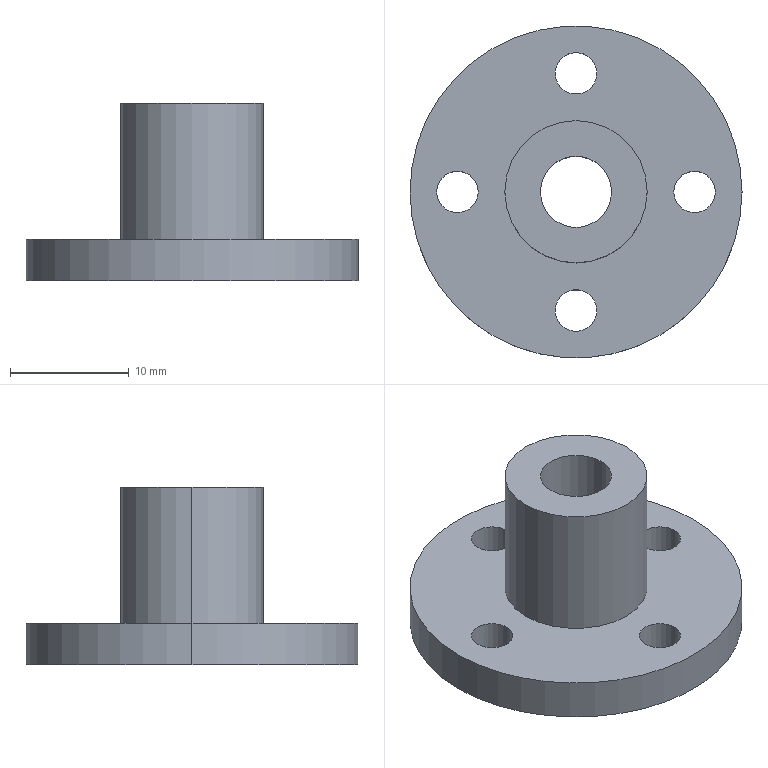Part | SolidWorks | features ICE 3, CirPattern 1, Extrusion 1 | 1 solid | 17 faces | box 28 x 28 x 15 mm | volume 2897 mm3 | cylinder 14 | plane 3 | commonest cylinder face diameters 3.5 x8 6 x2 12 x2 28 x2
STEP:
#1=CARTESIAN_POINT('',(-3.,0.,0.));
#2=VERTEX_POINT('',#1);
#3=CARTESIAN_POINT('',(3.,0.,0.));
#4=VERTEX_POINT('',#3);
#5=CARTESIAN_POINT('',(0.,0.,0.));
#6=DIRECTION('',(0.,0.,1.));
#7=DIRECTION('',(1.,0.,0.));
#8=AXIS2_PLACEMENT_3D('',#5,#6,#7);
#9=CIRCLE('',#8,3.);
#10=EDGE_CURVE('',#2,#4,#9,.T.);
#11=ORIENTED_EDGE('',*,*,#10,.F.);
#12=CARTESIAN_POINT('',(-3.,0.,15.));
#13=VERTEX_POINT('',#12);
#14=CARTESIAN_POINT('',(-3.,0.,-35.));
#15=DIRECTION('',(0.,0.,1.));
#16=VECTOR('',#15,1000.);
#17=LINE('',#14,#16);
#18=EDGE_CURVE('',#2,#13,#17,.T.);
#19=ORIENTED_EDGE('',*,*,#18,.T.);
#20=CARTESIAN_POINT('',(3.,0.,15.));
#21=VERTEX_POINT('',#20);
#22=CARTESIAN_POINT('',(0.,0.,15.));
#23=DIRECTION('',(0.,0.,1.));
#24=DIRECTION('',(1.,0.,0.));
#25=AXIS2_PLACEMENT_3D('',#22,#23,#24);
#26=CIRCLE('',#25,3.);
#27=EDGE_CURVE('',#13,#21,#26,.T.);
#28=ORIENTED_EDGE('',*,*,#27,.T.);
#29=CARTESIAN_POINT('',(3.,0.,-35.));
#30=DIRECTION('',(0.,0.,1.));
#31=VECTOR('',#30,1000.);
#32=LINE('',#29,#31);
#33=EDGE_CURVE('',#4,#21,#32,.T.);
#34=ORIENTED_EDGE('',*,*,#33,.F.);
#35=EDGE_LOOP('',(#11,#19,#28,#34));
#36=FACE_OUTER_BOUND('',#35,.T.);
#37=CARTESIAN_POINT('',(0.,0.,-35.));
#38=DIRECTION('',(0.,0.,1.));
#39=DIRECTION('',(1.,0.,0.));
#40=AXIS2_PLACEMENT_3D('',#37,#38,#39);
#41=CYLINDRICAL_SURFACE('',#40,3.);
#42=ADVANCED_FACE('',(#36),#41,.F.);
#43=CARTESIAN_POINT('',(-11.75,0.,0.));
#44=VERTEX_POINT('',#43);
#45=CARTESIAN_POINT('',(-8.25,0.,0.));
#46=VERTEX_POINT('',#45);
#47=CARTESIAN_POINT('',(-10.,0.,0.));
#48=DIRECTION('',(0.,0.,1.));
#49=DIRECTION('',(1.,0.,0.));
#50=AXIS2_PLACEMENT_3D('',#47,#48,#49);
#51=CIRCLE('',#50,1.75);
#52=EDGE_CURVE('',#44,#46,#51,.T.);
#53=ORIENTED_EDGE('',*,*,#52,.F.);
#54=CARTESIAN_POINT('',(-11.75,0.,3.5));
#55=VERTEX_POINT('',#54);
#56=CARTESIAN_POINT('',(-11.75,0.,-8.));
#57=DIRECTION('',(0.,0.,1.));
#58=VECTOR('',#57,1000.);
#59=LINE('',#56,#58);
#60=EDGE_CURVE('',#44,#55,#59,.T.);
#61=ORIENTED_EDGE('',*,*,#60,.T.);
#62=CARTESIAN_POINT('',(-8.25,0.,3.5));
#63=VERTEX_POINT('',#62);
#64=CARTESIAN_POINT('',(-10.,0.,3.5));
#65=DIRECTION('',(0.,0.,1.));
#66=DIRECTION('',(0.,1.,0.));
#67=AXIS2_PLACEMENT_3D('',#64,#65,#66);
#68=CIRCLE('',#67,1.75);
#69=EDGE_CURVE('',#55,#63,#68,.T.);
#70=ORIENTED_EDGE('',*,*,#69,.T.);
#71=CARTESIAN_POINT('',(-8.25,0.,-8.));
#72=DIRECTION('',(0.,0.,1.));
#73=VECTOR('',#72,1000.);
#74=LINE('',#71,#73);
#75=EDGE_CURVE('',#46,#63,#74,.T.);
#76=ORIENTED_EDGE('',*,*,#75,.F.);
#77=EDGE_LOOP('',(#53,#61,#70,#76));
#78=FACE_OUTER_BOUND('',#77,.T.);
#79=CARTESIAN_POINT('',(-10.,0.,-8.));
#80=DIRECTION('',(0.,0.,1.));
#81=DIRECTION('',(1.,0.,0.));
#82=AXIS2_PLACEMENT_3D('',#79,#80,#81);
#83=CYLINDRICAL_SURFACE('',#82,1.75);
#84=ADVANCED_FACE('',(#78),#83,.F.);
#85=CARTESIAN_POINT('',(-1.75,-10.,0.));
#86=VERTEX_POINT('',#85);
#87=CARTESIAN_POINT('',(1.75,-10.,0.));
#88=VERTEX_POINT('',#87);
#89=CARTESIAN_POINT('',(0.,-10.,0.));
#90=DIRECTION('',(0.,0.,1.));
#91=DIRECTION('',(1.,0.,0.));
#92=AXIS2_PLACEMENT_3D('',#89,#90,#91);
#93=CIRCLE('',#92,1.75);
#94=EDGE_CURVE('',#86,#88,#93,.T.);
#95=ORIENTED_EDGE('',*,*,#94,.F.);
#96=CARTESIAN_POINT('',(-1.75,-10.,3.5));
#97=VERTEX_POINT('',#96);
#98=CARTESIAN_POINT('',(-1.75,-10.,-8.));
#99=DIRECTION('',(0.,0.,1.));
#100=VECTOR('',#99,1000.);
#101=LINE('',#98,#100);
#102=EDGE_CURVE('',#86,#97,#101,.T.);
#103=ORIENTED_EDGE('',*,*,#102,.T.);
#104=CARTESIAN_POINT('',(1.75,-10.,3.5));
#105=VERTEX_POINT('',#104);
#106=CARTESIAN_POINT('',(0.,-10.,3.5));
#107=DIRECTION('',(0.,0.,1.));
#108=DIRECTION('',(-1.,0.,0.));
#109=AXIS2_PLACEMENT_3D('',#106,#107,#108);
#110=CIRCLE('',#109,1.75);
#111=EDGE_CURVE('',#97,#105,#110,.T.);
#112=ORIENTED_EDGE('',*,*,#111,.T.);
#113=CARTESIAN_POINT('',(1.75,-10.,-8.));
#114=DIRECTION('',(0.,0.,1.));
#115=VECTOR('',#114,1000.);
#116=LINE('',#113,#115);
#117=EDGE_CURVE('',#88,#105,#116,.T.);
#118=ORIENTED_EDGE('',*,*,#117,.F.);
#119=EDGE_LOOP('',(#95,#103,#112,#118));
#120=FACE_OUTER_BOUND('',#119,.T.);
#121=CARTESIAN_POINT('',(0.,-10.,-8.));
#122=DIRECTION('',(0.,0.,1.));
#123=DIRECTION('',(1.,0.,0.));
#124=AXIS2_PLACEMENT_3D('',#121,#122,#123);
#125=CYLINDRICAL_SURFACE('',#124,1.75);
#126=ADVANCED_FACE('',(#120),#125,.F.);
#127=CARTESIAN_POINT('',(8.25,0.,0.));
#128=VERTEX_POINT('',#127);
#129=CARTESIAN_POINT('',(11.75,0.,0.));
#130=VERTEX_POINT('',#129);
#131=CARTESIAN_POINT('',(10.,0.,0.));
#132=DIRECTION('',(0.,0.,1.));
#133=DIRECTION('',(1.,0.,0.));
#134=AXIS2_PLACEMENT_3D('',#131,#132,#133);
#135=CIRCLE('',#134,1.75);
#136=EDGE_CURVE('',#128,#130,#135,.T.);
#137=ORIENTED_EDGE('',*,*,#136,.F.);
#138=CARTESIAN_POINT('',(8.25,0.,3.5));
#139=VERTEX_POINT('',#138);
#140=CARTESIAN_POINT('',(8.25,0.,-8.));
#141=DIRECTION('',(0.,0.,1.));
#142=VECTOR('',#141,1000.);
#143=LINE('',#140,#142);
#144=EDGE_CURVE('',#128,#139,#143,.T.);
#145=ORIENTED_EDGE('',*,*,#144,.T.);
#146=CARTESIAN_POINT('',(11.75,0.,3.5));
#147=VERTEX_POINT('',#146);
#148=CARTESIAN_POINT('',(10.,0.,3.5));
#149=DIRECTION('',(0.,0.,1.));
#150=DIRECTION('',(0.,-1.,0.));
#151=AXIS2_PLACEMENT_3D('',#148,#149,#150);
#152=CIRCLE('',#151,1.75);
#153=EDGE_CURVE('',#139,#147,#152,.T.);
#154=ORIENTED_EDGE('',*,*,#153,.T.);
#155=CARTESIAN_POINT('',(11.75,0.,-8.));
#156=DIRECTION('',(0.,0.,1.));
#157=VECTOR('',#156,1000.);
#158=LINE('',#155,#157);
#159=EDGE_CURVE('',#130,#147,#158,.T.);
#160=ORIENTED_EDGE('',*,*,#159,.F.);
#161=EDGE_LOOP('',(#137,#145,#154,#160));
#162=FACE_OUTER_BOUND('',#161,.T.);
#163=CARTESIAN_POINT('',(10.,0.,-8.));
#164=DIRECTION('',(0.,0.,1.));
#165=DIRECTION('',(1.,0.,0.));
#166=AXIS2_PLACEMENT_3D('',#163,#164,#165);
#167=CYLINDRICAL_SURFACE('',#166,1.75);
#168=ADVANCED_FACE('',(#162),#167,.F.);
#169=CARTESIAN_POINT('',(-1.75,10.,0.));
#170=VERTEX_POINT('',#169);
#171=CARTESIAN_POINT('',(1.75,10.,0.));
#172=VERTEX_POINT('',#171);
#173=CARTESIAN_POINT('',(0.,10.,0.));
#174=DIRECTION('',(0.,0.,1.));
#175=DIRECTION('',(1.,0.,0.));
#176=AXIS2_PLACEMENT_3D('',#173,#174,#175);
#177=CIRCLE('',#176,1.75);
#178=EDGE_CURVE('',#170,#172,#177,.T.);
#179=ORIENTED_EDGE('',*,*,#178,.F.);
#180=CARTESIAN_POINT('',(-1.75,10.,3.5));
#181=VERTEX_POINT('',#180);
#182=CARTESIAN_POINT('',(-1.75,10.,-8.));
#183=DIRECTION('',(0.,0.,1.));
#184=VECTOR('',#183,1000.);
#185=LINE('',#182,#184);
#186=EDGE_CURVE('',#170,#181,#185,.T.);
#187=ORIENTED_EDGE('',*,*,#186,.T.);
#188=CARTESIAN_POINT('',(1.75,10.,3.5));
#189=VERTEX_POINT('',#188);
#190=CARTESIAN_POINT('',(0.,10.,3.5));
#191=DIRECTION('',(0.,0.,1.));
#192=DIRECTION('',(1.,0.,0.));
#193=AXIS2_PLACEMENT_3D('',#190,#191,#192);
#194=CIRCLE('',#193,1.75);
#195=EDGE_CURVE('',#181,#189,#194,.T.);
#196=ORIENTED_EDGE('',*,*,#195,.T.);
#197=CARTESIAN_POINT('',(1.75,10.,-8.));
#198=DIRECTION('',(0.,0.,1.));
#199=VECTOR('',#198,1000.);
#200=LINE('',#197,#199);
#201=EDGE_CURVE('',#172,#189,#200,.T.);
#202=ORIENTED_EDGE('',*,*,#201,.F.);
#203=EDGE_LOOP('',(#179,#187,#196,#202));
#204=FACE_OUTER_BOUND('',#203,.T.);
#205=CARTESIAN_POINT('',(0.,10.,-8.));
#206=DIRECTION('',(0.,0.,1.));
#207=DIRECTION('',(1.,0.,0.));
#208=AXIS2_PLACEMENT_3D('',#205,#206,#207);
#209=CYLINDRICAL_SURFACE('',#208,1.75);
#210=ADVANCED_FACE('',(#204),#209,.F.);
#211=CARTESIAN_POINT('',(6.,0.,15.));
#212=VERTEX_POINT('',#211);
#213=CARTESIAN_POINT('',(-6.,0.,15.));
#214=VERTEX_POINT('',#213);
#215=CARTESIAN_POINT('',(0.,0.,15.));
#216=DIRECTION('',(0.,0.,1.));
#217=DIRECTION('',(1.,0.,0.));
#218=AXIS2_PLACEMENT_3D('',#215,#216,#217);
#219=CIRCLE('',#218,6.);
#220=EDGE_CURVE('',#212,#214,#219,.T.);
#221=ORIENTED_EDGE('',*,*,#220,.F.);
#222=CARTESIAN_POINT('',(6.,0.,3.5));
#223=VERTEX_POINT('',#222);
#224=CARTESIAN_POINT('',(6.,0.,15.));
#225=DIRECTION('',(0.,0.,-1.));
#226=VECTOR('',#225,1000.);
#227=LINE('',#224,#226);
#228=EDGE_CURVE('',#212,#223,#227,.T.);
#229=ORIENTED_EDGE('',*,*,#228,.T.);
#230=CARTESIAN_POINT('',(-6.,0.,3.5));
#231=VERTEX_POINT('',#230);
#232=CARTESIAN_POINT('',(0.,0.,3.5));
#233=DIRECTION('',(0.,0.,1.));
#234=DIRECTION('',(1.,0.,0.));
#235=AXIS2_PLACEMENT_3D('',#232,#233,#234);
#236=CIRCLE('',#235,6.);
#237=EDGE_CURVE('',#223,#231,#236,.T.);
#238=ORIENTED_EDGE('',*,*,#237,.T.);
#239=CARTESIAN_POINT('',(-6.,0.,15.));
#240=DIRECTION('',(0.,0.,-1.));
#241=VECTOR('',#240,1000.);
#242=LINE('',#239,#241);
#243=EDGE_CURVE('',#214,#231,#242,.T.);
#244=ORIENTED_EDGE('',*,*,#243,.F.);
#245=EDGE_LOOP('',(#221,#229,#238,#244));
#246=FACE_OUTER_BOUND('',#245,.T.);
#247=CARTESIAN_POINT('',(0.,0.,15.));
#248=DIRECTION('',(0.,0.,-1.));
#249=DIRECTION('',(-1.,0.,0.));
#250=AXIS2_PLACEMENT_3D('',#247,#248,#249);
#251=CYLINDRICAL_SURFACE('',#250,6.);
#252=ADVANCED_FACE('',(#246),#251,.T.);
#253=CARTESIAN_POINT('',(14.,0.,3.5));
#254=VERTEX_POINT('',#253);
#255=CARTESIAN_POINT('',(-14.,0.,3.5));
#256=VERTEX_POINT('',#255);
#257=CARTESIAN_POINT('',(0.,0.,3.5));
#258=DIRECTION('',(0.,0.,1.));
#259=DIRECTION('',(1.,0.,0.));
#260=AXIS2_PLACEMENT_3D('',#257,#258,#259);
#261=CIRCLE('',#260,14.);
#262=EDGE_CURVE('',#254,#256,#261,.T.);
#263=ORIENTED_EDGE('',*,*,#262,.F.);
#264=CARTESIAN_POINT('',(14.,0.,0.));
#265=VERTEX_POINT('',#264);
#266=CARTESIAN_POINT('',(14.,0.,3.5));
#267=DIRECTION('',(0.,0.,-1.));
#268=VECTOR('',#267,1000.);
#269=LINE('',#266,#268);
#270=EDGE_CURVE('',#254,#265,#269,.T.);
#271=ORIENTED_EDGE('',*,*,#270,.T.);
#272=CARTESIAN_POINT('',(-14.,0.,0.));
#273=VERTEX_POINT('',#272);
#274=CARTESIAN_POINT('',(0.,0.,0.));
#275=DIRECTION('',(0.,0.,1.));
#276=DIRECTION('',(1.,0.,0.));
#277=AXIS2_PLACEMENT_3D('',#274,#275,#276);
#278=CIRCLE('',#277,14.);
#279=EDGE_CURVE('',#265,#273,#278,.T.);
#280=ORIENTED_EDGE('',*,*,#279,.T.);
#281=CARTESIAN_POINT('',(-14.,0.,3.5));
#282=DIRECTION('',(0.,0.,-1.));
#283=VECTOR('',#282,1000.);
#284=LINE('',#281,#283);
#285=EDGE_CURVE('',#256,#273,#284,.T.);
#286=ORIENTED_EDGE('',*,*,#285,.F.);
#287=EDGE_LOOP('',(#263,#271,#280,#286));
#288=FACE_OUTER_BOUND('',#287,.T.);
#289=CARTESIAN_POINT('',(0.,0.,3.5));
#290=DIRECTION('',(0.,0.,-1.));
#291=DIRECTION('',(-1.,0.,0.));
#292=AXIS2_PLACEMENT_3D('',#289,#290,#291);
#293=CYLINDRICAL_SURFACE('',#292,14.);
#294=ADVANCED_FACE('',(#288),#293,.T.);
#295=ORIENTED_EDGE('',*,*,#270,.F.);
#296=CARTESIAN_POINT('',(0.,0.,3.5));
#297=DIRECTION('',(0.,0.,1.));
#298=DIRECTION('',(1.,0.,0.));
#299=AXIS2_PLACEMENT_3D('',#296,#297,#298);
#300=CIRCLE('',#299,14.);
#301=EDGE_CURVE('',#256,#254,#300,.T.);
#302=ORIENTED_EDGE('',*,*,#301,.F.);
#303=ORIENTED_EDGE('',*,*,#285,.T.);
#304=CARTESIAN_POINT('',(0.,0.,0.));
#305=DIRECTION('',(0.,0.,1.));
#306=DIRECTION('',(1.,0.,0.));
#307=AXIS2_PLACEMENT_3D('',#304,#305,#306);
#308=CIRCLE('',#307,14.);
#309=EDGE_CURVE('',#273,#265,#308,.T.);
#310=ORIENTED_EDGE('',*,*,#309,.T.);
#311=EDGE_LOOP('',(#295,#302,#303,#310));
#312=FACE_OUTER_BOUND('',#311,.T.);
#313=CARTESIAN_POINT('',(0.,0.,3.5));
#314=DIRECTION('',(0.,0.,-1.));
#315=DIRECTION('',(-1.,0.,0.));
#316=AXIS2_PLACEMENT_3D('',#313,#314,#315);
#317=CYLINDRICAL_SURFACE('',#316,14.);
#318=ADVANCED_FACE('',(#312),#317,.T.);
#319=CARTESIAN_POINT('',(-10.,0.,3.5));
#320=DIRECTION('',(0.,0.,1.));
#321=DIRECTION('',(0.,1.,0.));
#322=AXIS2_PLACEMENT_3D('',#319,#320,#321);
#323=CIRCLE('',#322,1.75);
#324=EDGE_CURVE('',#63,#55,#323,.T.);
#325=ORIENTED_EDGE('',*,*,#324,.F.);
#326=ORIENTED_EDGE('',*,*,#69,.F.);
#327=EDGE_LOOP('',(#325,#326));
#328=FACE_BOUND('',#327,.T.);
#329=CARTESIAN_POINT('',(0.,-10.,3.5));
#330=DIRECTION('',(0.,0.,1.));
#331=DIRECTION('',(-1.,0.,0.));
#332=AXIS2_PLACEMENT_3D('',#329,#330,#331);
#333=CIRCLE('',#332,1.75);
#334=EDGE_CURVE('',#105,#97,#333,.T.);
#335=ORIENTED_EDGE('',*,*,#334,.F.);
#336=ORIENTED_EDGE('',*,*,#111,.F.);
#337=EDGE_LOOP('',(#335,#336));
#338=FACE_BOUND('',#337,.T.);
#339=CARTESIAN_POINT('',(10.,0.,3.5));
#340=DIRECTION('',(0.,0.,1.));
#341=DIRECTION('',(0.,-1.,0.));
#342=AXIS2_PLACEMENT_3D('',#339,#340,#341);
#343=CIRCLE('',#342,1.75);
#344=EDGE_CURVE('',#147,#139,#343,.T.);
#345=ORIENTED_EDGE('',*,*,#344,.F.);
#346=ORIENTED_EDGE('',*,*,#153,.F.);
#347=EDGE_LOOP('',(#345,#346));
#348=FACE_BOUND('',#347,.T.);
#349=CARTESIAN_POINT('',(0.,10.,3.5));
#350=DIRECTION('',(0.,0.,1.));
#351=DIRECTION('',(1.,0.,0.));
#352=AXIS2_PLACEMENT_3D('',#349,#350,#351);
#353=CIRCLE('',#352,1.75);
#354=EDGE_CURVE('',#189,#181,#353,.T.);
#355=ORIENTED_EDGE('',*,*,#354,.F.);
#356=ORIENTED_EDGE('',*,*,#195,.F.);
#357=EDGE_LOOP('',(#355,#356));
#358=FACE_BOUND('',#357,.T.);
#359=CARTESIAN_POINT('',(0.,0.,3.5));
#360=DIRECTION('',(0.,0.,1.));
#361=DIRECTION('',(1.,0.,0.));
#362=AXIS2_PLACEMENT_3D('',#359,#360,#361);
#363=CIRCLE('',#362,6.);
#364=EDGE_CURVE('',#231,#223,#363,.T.);
#365=ORIENTED_EDGE('',*,*,#364,.F.);
#366=ORIENTED_EDGE('',*,*,#237,.F.);
#367=EDGE_LOOP('',(#365,#366));
#368=FACE_BOUND('',#367,.T.);
#369=ORIENTED_EDGE('',*,*,#301,.T.);
#370=ORIENTED_EDGE('',*,*,#262,.T.);
#371=EDGE_LOOP('',(#369,#370));
#372=FACE_OUTER_BOUND('',#371,.T.);
#373=CARTESIAN_POINT('',(0.,0.,3.5));
#374=DIRECTION('',(0.,0.,1.));
#375=DIRECTION('',(1.,0.,0.));
#376=AXIS2_PLACEMENT_3D('',#373,#374,#375);
#377=PLANE('',#376);
#378=ADVANCED_FACE('',(#328,#338,#348,#358,#368,#372),#377,.T.);
#379=CARTESIAN_POINT('',(0.,0.,0.));
#380=DIRECTION('',(0.,0.,1.));
#381=DIRECTION('',(1.,0.,0.));
#382=AXIS2_PLACEMENT_3D('',#379,#380,#381);
#383=CIRCLE('',#382,3.);
#384=EDGE_CURVE('',#4,#2,#383,.T.);
#385=ORIENTED_EDGE('',*,*,#384,.T.);
#386=ORIENTED_EDGE('',*,*,#10,.T.);
#387=EDGE_LOOP('',(#385,#386));
#388=FACE_BOUND('',#387,.T.);
#389=CARTESIAN_POINT('',(-10.,0.,0.));
#390=DIRECTION('',(0.,0.,1.));
#391=DIRECTION('',(1.,0.,0.));
#392=AXIS2_PLACEMENT_3D('',#389,#390,#391);
#393=CIRCLE('',#392,1.75);
#394=EDGE_CURVE('',#46,#44,#393,.T.);
#395=ORIENTED_EDGE('',*,*,#394,.T.);
#396=ORIENTED_EDGE('',*,*,#52,.T.);
#397=EDGE_LOOP('',(#395,#396));
#398=FACE_BOUND('',#397,.T.);
#399=CARTESIAN_POINT('',(0.,-10.,0.));
#400=DIRECTION('',(0.,0.,1.));
#401=DIRECTION('',(1.,0.,0.));
#402=AXIS2_PLACEMENT_3D('',#399,#400,#401);
#403=CIRCLE('',#402,1.75);
#404=EDGE_CURVE('',#88,#86,#403,.T.);
#405=ORIENTED_EDGE('',*,*,#404,.T.);
#406=ORIENTED_EDGE('',*,*,#94,.T.);
#407=EDGE_LOOP('',(#405,#406));
#408=FACE_BOUND('',#407,.T.);
#409=CARTESIAN_POINT('',(10.,0.,0.));
#410=DIRECTION('',(0.,0.,1.));
#411=DIRECTION('',(1.,0.,0.));
#412=AXIS2_PLACEMENT_3D('',#409,#410,#411);
#413=CIRCLE('',#412,1.75);
#414=EDGE_CURVE('',#130,#128,#413,.T.);
#415=ORIENTED_EDGE('',*,*,#414,.T.);
#416=ORIENTED_EDGE('',*,*,#136,.T.);
#417=EDGE_LOOP('',(#415,#416));
#418=FACE_BOUND('',#417,.T.);
#419=CARTESIAN_POINT('',(0.,10.,0.));
#420=DIRECTION('',(0.,0.,1.));
#421=DIRECTION('',(1.,0.,0.));
#422=AXIS2_PLACEMENT_3D('',#419,#420,#421);
#423=CIRCLE('',#422,1.75);
#424=EDGE_CURVE('',#172,#170,#423,.T.);
#425=ORIENTED_EDGE('',*,*,#424,.T.);
#426=ORIENTED_EDGE('',*,*,#178,.T.);
#427=EDGE_LOOP('',(#425,#426));
#428=FACE_BOUND('',#427,.T.);
#429=ORIENTED_EDGE('',*,*,#309,.F.);
#430=ORIENTED_EDGE('',*,*,#279,.F.);
#431=EDGE_LOOP('',(#429,#430));
#432=FACE_OUTER_BOUND('',#431,.T.);
#433=CARTESIAN_POINT('',(0.,0.,0.));
#434=DIRECTION('',(0.,0.,1.));
#435=DIRECTION('',(1.,0.,0.));
#436=AXIS2_PLACEMENT_3D('',#433,#434,#435);
#437=PLANE('',#436);
#438=ADVANCED_FACE('',(#388,#398,#408,#418,#428,#432),#437,.F.);
#439=ORIENTED_EDGE('',*,*,#228,.F.);
#440=CARTESIAN_POINT('',(0.,0.,15.));
#441=DIRECTION('',(0.,0.,1.));
#442=DIRECTION('',(1.,0.,0.));
#443=AXIS2_PLACEMENT_3D('',#440,#441,#442);
#444=CIRCLE('',#443,6.);
#445=EDGE_CURVE('',#214,#212,#444,.T.);
#446=ORIENTED_EDGE('',*,*,#445,.F.);
#447=ORIENTED_EDGE('',*,*,#243,.T.);
#448=ORIENTED_EDGE('',*,*,#364,.T.);
#449=EDGE_LOOP('',(#439,#446,#447,#448));
#450=FACE_OUTER_BOUND('',#449,.T.);
#451=CARTESIAN_POINT('',(0.,0.,15.));
#452=DIRECTION('',(0.,0.,-1.));
#453=DIRECTION('',(-1.,0.,0.));
#454=AXIS2_PLACEMENT_3D('',#451,#452,#453);
#455=CYLINDRICAL_SURFACE('',#454,6.);
#456=ADVANCED_FACE('',(#450),#455,.T.);
#457=CARTESIAN_POINT('',(0.,0.,15.));
#458=DIRECTION('',(0.,0.,1.));
#459=DIRECTION('',(1.,0.,0.));
#460=AXIS2_PLACEMENT_3D('',#457,#458,#459);
#461=CIRCLE('',#460,3.);
#462=EDGE_CURVE('',#21,#13,#461,.T.);
#463=ORIENTED_EDGE('',*,*,#462,.F.);
#464=ORIENTED_EDGE('',*,*,#27,.F.);
#465=EDGE_LOOP('',(#463,#464));
#466=FACE_BOUND('',#465,.T.);
#467=ORIENTED_EDGE('',*,*,#445,.T.);
#468=ORIENTED_EDGE('',*,*,#220,.T.);
#469=EDGE_LOOP('',(#467,#468));
#470=FACE_OUTER_BOUND('',#469,.T.);
#471=CARTESIAN_POINT('',(0.,0.,15.));
#472=DIRECTION('',(0.,0.,1.));
#473=DIRECTION('',(1.,0.,0.));
#474=AXIS2_PLACEMENT_3D('',#471,#472,#473);
#475=PLANE('',#474);
#476=ADVANCED_FACE('',(#466,#470),#475,.T.);
#477=ORIENTED_EDGE('',*,*,#186,.F.);
#478=ORIENTED_EDGE('',*,*,#424,.F.);
#479=ORIENTED_EDGE('',*,*,#201,.T.);
#480=ORIENTED_EDGE('',*,*,#354,.T.);
#481=EDGE_LOOP('',(#477,#478,#479,#480));
#482=FACE_OUTER_BOUND('',#481,.T.);
#483=CARTESIAN_POINT('',(0.,10.,-8.));
#484=DIRECTION('',(0.,0.,1.));
#485=DIRECTION('',(1.,0.,0.));
#486=AXIS2_PLACEMENT_3D('',#483,#484,#485);
#487=CYLINDRICAL_SURFACE('',#486,1.75);
#488=ADVANCED_FACE('',(#482),#487,.F.);
#489=ORIENTED_EDGE('',*,*,#144,.F.);
#490=ORIENTED_EDGE('',*,*,#414,.F.);
#491=ORIENTED_EDGE('',*,*,#159,.T.);
#492=ORIENTED_EDGE('',*,*,#344,.T.);
#493=EDGE_LOOP('',(#489,#490,#491,#492));
#494=FACE_OUTER_BOUND('',#493,.T.);
#495=CARTESIAN_POINT('',(10.,0.,-8.));
#496=DIRECTION('',(0.,0.,1.));
#497=DIRECTION('',(1.,0.,0.));
#498=AXIS2_PLACEMENT_3D('',#495,#496,#497);
#499=CYLINDRICAL_SURFACE('',#498,1.75);
#500=ADVANCED_FACE('',(#494),#499,.F.);
#501=ORIENTED_EDGE('',*,*,#102,.F.);
#502=ORIENTED_EDGE('',*,*,#404,.F.);
#503=ORIENTED_EDGE('',*,*,#117,.T.);
#504=ORIENTED_EDGE('',*,*,#334,.T.);
#505=EDGE_LOOP('',(#501,#502,#503,#504));
#506=FACE_OUTER_BOUND('',#505,.T.);
#507=CARTESIAN_POINT('',(0.,-10.,-8.));
#508=DIRECTION('',(0.,0.,1.));
#509=DIRECTION('',(1.,0.,0.));
#510=AXIS2_PLACEMENT_3D('',#507,#508,#509);
#511=CYLINDRICAL_SURFACE('',#510,1.75);
#512=ADVANCED_FACE('',(#506),#511,.F.);
#513=ORIENTED_EDGE('',*,*,#60,.F.);
#514=ORIENTED_EDGE('',*,*,#394,.F.);
#515=ORIENTED_EDGE('',*,*,#75,.T.);
#516=ORIENTED_EDGE('',*,*,#324,.T.);
#517=EDGE_LOOP('',(#513,#514,#515,#516));
#518=FACE_OUTER_BOUND('',#517,.T.);
#519=CARTESIAN_POINT('',(-10.,0.,-8.));
#520=DIRECTION('',(0.,0.,1.));
#521=DIRECTION('',(1.,0.,0.));
#522=AXIS2_PLACEMENT_3D('',#519,#520,#521);
#523=CYLINDRICAL_SURFACE('',#522,1.75);
#524=ADVANCED_FACE('',(#518),#523,.F.);
#525=ORIENTED_EDGE('',*,*,#18,.F.);
#526=ORIENTED_EDGE('',*,*,#384,.F.);
#527=ORIENTED_EDGE('',*,*,#33,.T.);
#528=ORIENTED_EDGE('',*,*,#462,.T.);
#529=EDGE_LOOP('',(#525,#526,#527,#528));
#530=FACE_OUTER_BOUND('',#529,.T.);
#531=CARTESIAN_POINT('',(0.,0.,-35.));
#532=DIRECTION('',(0.,0.,1.));
#533=DIRECTION('',(1.,0.,0.));
#534=AXIS2_PLACEMENT_3D('',#531,#532,#533);
#535=CYLINDRICAL_SURFACE('',#534,3.);
#536=ADVANCED_FACE('',(#530),#535,.F.);
#537=CLOSED_SHELL('',(#42,#84,#126,#168,#210,#252,#294,#318,#378,#438,#456,#476,#488,#500,#512,#524,#536));
#538=MANIFOLD_SOLID_BREP('',#537);
#539=CARTESIAN_POINT('',(0.,0.,0.));
#540=DIRECTION('',(0.,0.,1.));
#541=DIRECTION('',(1.,0.,0.));
#542=AXIS2_PLACEMENT_3D('',#539,#540,#541);
#543=(LENGTH_UNIT()NAMED_UNIT(*)SI_UNIT(.MILLI.,.METRE.));
#544=UNCERTAINTY_MEASURE_WITH_UNIT(LENGTH_MEASURE(0.00001),#543,'','');
#545=(NAMED_UNIT(*)PLANE_ANGLE_UNIT()SI_UNIT($,.RADIAN.));
#546=(NAMED_UNIT(*)SI_UNIT($,.STERADIAN.)SOLID_ANGLE_UNIT());
#547=(GEOMETRIC_REPRESENTATION_CONTEXT(3)GLOBAL_UNCERTAINTY_ASSIGNED_CONTEXT((#544))GLOBAL_UNIT_ASSIGNED_CONTEXT((#543,#545,#546))REPRESENTATION_CONTEXT('',''));
#548=ADVANCED_BREP_SHAPE_REPRESENTATION('',(#538,#542),#547);